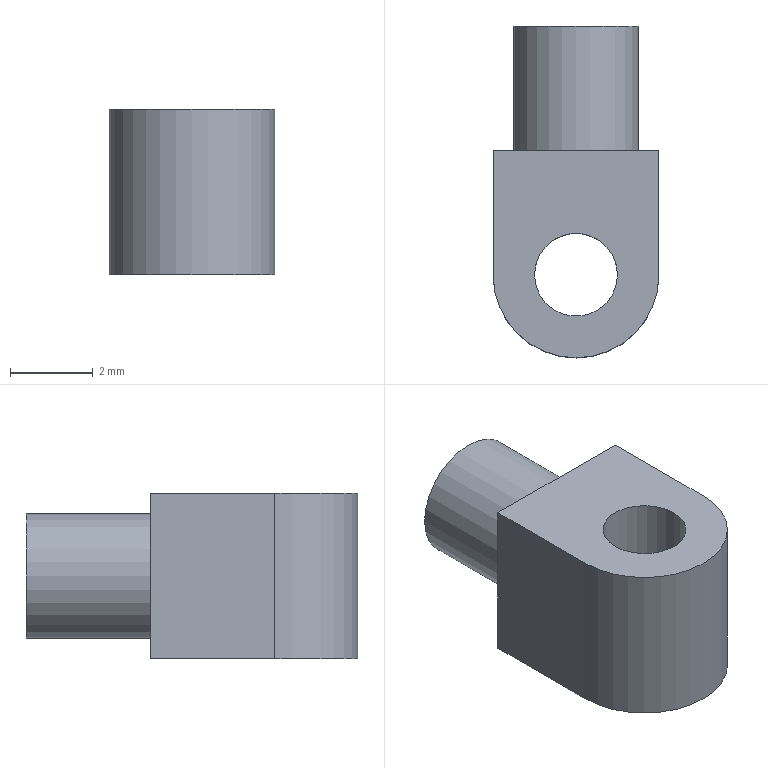Part | STEP file | 1-56.20 | 1 solid | 9 faces | box 4 x 8 x 4 mm | volume 81.772 mm3 | plane 6 | cylinder 3 | commonest cylinder face diameters 2 x1 3 x1 4 x1
STEP:
#1=CARTESIAN_POINT('',(0.,0.,0.));
#2=DIRECTION('',(0.,0.,1.));
#3=DIRECTION('',(1.,0.,0.));
#4=AXIS2_PLACEMENT_3D('',#1,#2,#3);
#5=CARTESIAN_POINT('',(1.5,3.,0.));
#6=VERTEX_POINT('',#5);
#7=CARTESIAN_POINT('',(0.,3.,0.));
#8=DIRECTION('',(0.,-1.,0.));
#9=DIRECTION('',(1.,0.,0.));
#10=AXIS2_PLACEMENT_3D('',#7,#8,#9);
#11=CIRCLE('',#10,1.5);
#12=CARTESIAN_POINT('',(-0.4019,3.,0.));
#13=DIRECTION('',(0.,-1.,0.));
#14=DIRECTION('',(1.,0.,0.));
#15=AXIS2_PLACEMENT_3D('',#12,#13,#14);
#16=PLANE('',#15);
#17=CARTESIAN_POINT('',(0.4019,0.));
#18=DIRECTION('',(1.,0.));
#19=AXIS2_PLACEMENT_2D('',#17,#18);
#20=CIRCLE('',#19,1.5);
#21=(GEOMETRIC_REPRESENTATION_CONTEXT(2)PARAMETRIC_REPRESENTATION_CONTEXT()REPRESENTATION_CONTEXT('',''));
#22=DEFINITIONAL_REPRESENTATION('',(#20),#21);
#23=PCURVE('',#16,#22);
#24=CARTESIAN_POINT('',(0.,0.,0.));
#25=DIRECTION('',(0.,1.,0.));
#26=DIRECTION('',(1.,0.,0.));
#27=AXIS2_PLACEMENT_3D('',#24,#25,#26);
#28=CYLINDRICAL_SURFACE('',#27,1.5);
#29=CARTESIAN_POINT('',(6.283,3.));
#30=DIRECTION('',(-1.,0.));
#31=VECTOR('',#30,1.);
#32=LINE('',#29,#31);
#33=(GEOMETRIC_REPRESENTATION_CONTEXT(2)PARAMETRIC_REPRESENTATION_CONTEXT()REPRESENTATION_CONTEXT('',''));
#34=DEFINITIONAL_REPRESENTATION('',(#32),#33);
#35=PCURVE('',#28,#34);
#36=SURFACE_CURVE('',#11,(#23,#35),.PCURVE_S1.);
#37=EDGE_CURVE('',#6,#6,#36,.T.);
#38=ORIENTED_EDGE('',*,*,#37,.T.);
#39=EDGE_LOOP('',(#38));
#40=FACE_BOUND('',#39,.F.);
#41=ADVANCED_FACE('',(#40),#16,.F.);
#42=CARTESIAN_POINT('',(1.5,0.,0.));
#43=VERTEX_POINT('',#42);
#44=CARTESIAN_POINT('',(1.5,0.,0.));
#45=DIRECTION('',(0.,1.,0.));
#46=VECTOR('',#45,1.);
#47=LINE('',#44,#46);
#48=CARTESIAN_POINT('',(6.283,0.));
#49=DIRECTION('',(0.,1.));
#50=VECTOR('',#49,1.);
#51=LINE('',#48,#50);
#52=(GEOMETRIC_REPRESENTATION_CONTEXT(2)PARAMETRIC_REPRESENTATION_CONTEXT()REPRESENTATION_CONTEXT('',''));
#53=DEFINITIONAL_REPRESENTATION('',(#51),#52);
#54=PCURVE('',#28,#53);
#55=CARTESIAN_POINT('',(0.,0.));
#56=DIRECTION('',(0.,1.));
#57=VECTOR('',#56,1.);
#58=LINE('',#55,#57);
#59=(GEOMETRIC_REPRESENTATION_CONTEXT(2)PARAMETRIC_REPRESENTATION_CONTEXT()REPRESENTATION_CONTEXT('',''));
#60=DEFINITIONAL_REPRESENTATION('',(#58),#59);
#61=PCURVE('',#28,#60);
#62=SEAM_CURVE('',#47,(#54,#61),.PCURVE_S1.);
#63=EDGE_CURVE('',#43,#6,#62,.T.);
#64=ORIENTED_EDGE('',*,*,#63,.T.);
#65=ORIENTED_EDGE('',*,*,#37,.T.);
#66=ORIENTED_EDGE('',*,*,#63,.F.);
#67=CARTESIAN_POINT('',(0.,0.,0.));
#68=DIRECTION('',(0.,-1.,0.));
#69=DIRECTION('',(1.,0.,0.));
#70=AXIS2_PLACEMENT_3D('',#67,#68,#69);
#71=CIRCLE('',#70,1.5);
#72=CARTESIAN_POINT('',(6.283,0.));
#73=DIRECTION('',(-1.,0.));
#74=VECTOR('',#73,1.);
#75=LINE('',#72,#74);
#76=(GEOMETRIC_REPRESENTATION_CONTEXT(2)PARAMETRIC_REPRESENTATION_CONTEXT()REPRESENTATION_CONTEXT('',''));
#77=DEFINITIONAL_REPRESENTATION('',(#75),#76);
#78=PCURVE('',#28,#77);
#79=CARTESIAN_POINT('',(0.,0.,0.));
#80=DIRECTION('',(0.,-1.,0.));
#81=DIRECTION('',(-1.,0.,0.));
#82=AXIS2_PLACEMENT_3D('',#79,#80,#81);
#83=PLANE('',#82);
#84=CARTESIAN_POINT('',(0.,0.));
#85=DIRECTION('',(-1.,0.));
#86=AXIS2_PLACEMENT_2D('',#84,#85);
#87=CIRCLE('',#86,1.5);
#88=(GEOMETRIC_REPRESENTATION_CONTEXT(2)PARAMETRIC_REPRESENTATION_CONTEXT()REPRESENTATION_CONTEXT('',''));
#89=DEFINITIONAL_REPRESENTATION('',(#87),#88);
#90=PCURVE('',#83,#89);
#91=SURFACE_CURVE('',#71,(#78,#90),.PCURVE_S1.);
#92=EDGE_CURVE('',#43,#43,#91,.T.);
#93=ORIENTED_EDGE('',*,*,#92,.F.);
#94=EDGE_LOOP('',(#64,#65,#66,#93));
#95=FACE_BOUND('',#94,.T.);
#96=ADVANCED_FACE('',(#95),#28,.T.);
#97=CARTESIAN_POINT('',(2.,0.,2.));
#98=VERTEX_POINT('',#97);
#99=CARTESIAN_POINT('',(-2.,0.,2.));
#100=VERTEX_POINT('',#99);
#101=CARTESIAN_POINT('',(2.,0.,2.));
#102=DIRECTION('',(-1.,0.,0.));
#103=VECTOR('',#102,1.);
#104=LINE('',#101,#103);
#105=CARTESIAN_POINT('',(-2.,-2.));
#106=DIRECTION('',(1.,0.));
#107=VECTOR('',#106,1.);
#108=LINE('',#105,#107);
#109=(GEOMETRIC_REPRESENTATION_CONTEXT(2)PARAMETRIC_REPRESENTATION_CONTEXT()REPRESENTATION_CONTEXT('',''));
#110=DEFINITIONAL_REPRESENTATION('',(#108),#109);
#111=PCURVE('',#83,#110);
#112=CARTESIAN_POINT('',(0.5,-2.5,2.));
#113=DIRECTION('',(0.,0.,1.));
#114=DIRECTION('',(1.,0.,0.));
#115=AXIS2_PLACEMENT_3D('',#112,#113,#114);
#116=PLANE('',#115);
#117=CARTESIAN_POINT('',(1.5,2.5));
#118=DIRECTION('',(-1.,0.));
#119=VECTOR('',#118,1.);
#120=LINE('',#117,#119);
#121=(GEOMETRIC_REPRESENTATION_CONTEXT(2)PARAMETRIC_REPRESENTATION_CONTEXT()REPRESENTATION_CONTEXT('',''));
#122=DEFINITIONAL_REPRESENTATION('',(#120),#121);
#123=PCURVE('',#116,#122);
#124=SURFACE_CURVE('',#104,(#111,#123),.PCURVE_S1.);
#125=EDGE_CURVE('',#98,#100,#124,.T.);
#126=ORIENTED_EDGE('',*,*,#125,.T.);
#127=CARTESIAN_POINT('',(-2.,0.,-2.));
#128=VERTEX_POINT('',#127);
#129=CARTESIAN_POINT('',(-2.,0.,2.));
#130=DIRECTION('',(0.,0.,-1.));
#131=VECTOR('',#130,1.);
#132=LINE('',#129,#131);
#133=CARTESIAN_POINT('',(2.,-2.));
#134=DIRECTION('',(0.,1.));
#135=VECTOR('',#134,1.);
#136=LINE('',#133,#135);
#137=(GEOMETRIC_REPRESENTATION_CONTEXT(2)PARAMETRIC_REPRESENTATION_CONTEXT()REPRESENTATION_CONTEXT('',''));
#138=DEFINITIONAL_REPRESENTATION('',(#136),#137);
#139=PCURVE('',#83,#138);
#140=CARTESIAN_POINT('',(-2.,-1.5,0.));
#141=DIRECTION('',(1.,0.,0.));
#142=DIRECTION('',(0.,-1.,0.));
#143=AXIS2_PLACEMENT_3D('',#140,#141,#142);
#144=PLANE('',#143);
#145=CARTESIAN_POINT('',(-1.5,-2.));
#146=DIRECTION('',(0.,1.));
#147=VECTOR('',#146,1.);
#148=LINE('',#145,#147);
#149=(GEOMETRIC_REPRESENTATION_CONTEXT(2)PARAMETRIC_REPRESENTATION_CONTEXT()REPRESENTATION_CONTEXT('',''));
#150=DEFINITIONAL_REPRESENTATION('',(#148),#149);
#151=PCURVE('',#144,#150);
#152=SURFACE_CURVE('',#132,(#139,#151),.PCURVE_S1.);
#153=EDGE_CURVE('',#100,#128,#152,.T.);
#154=ORIENTED_EDGE('',*,*,#153,.T.);
#155=CARTESIAN_POINT('',(2.,0.,-2.));
#156=VERTEX_POINT('',#155);
#157=CARTESIAN_POINT('',(2.,0.,-2.));
#158=DIRECTION('',(-1.,0.,0.));
#159=VECTOR('',#158,1.);
#160=LINE('',#157,#159);
#161=CARTESIAN_POINT('',(-2.,2.));
#162=DIRECTION('',(1.,0.));
#163=VECTOR('',#162,1.);
#164=LINE('',#161,#163);
#165=(GEOMETRIC_REPRESENTATION_CONTEXT(2)PARAMETRIC_REPRESENTATION_CONTEXT()REPRESENTATION_CONTEXT('',''));
#166=DEFINITIONAL_REPRESENTATION('',(#164),#165);
#167=PCURVE('',#83,#166);
#168=CARTESIAN_POINT('',(0.5,-2.5,-2.));
#169=DIRECTION('',(0.,0.,1.));
#170=DIRECTION('',(1.,0.,0.));
#171=AXIS2_PLACEMENT_3D('',#168,#169,#170);
#172=PLANE('',#171);
#173=CARTESIAN_POINT('',(1.5,2.5));
#174=DIRECTION('',(-1.,0.));
#175=VECTOR('',#174,1.);
#176=LINE('',#173,#175);
#177=(GEOMETRIC_REPRESENTATION_CONTEXT(2)PARAMETRIC_REPRESENTATION_CONTEXT()REPRESENTATION_CONTEXT('',''));
#178=DEFINITIONAL_REPRESENTATION('',(#176),#177);
#179=PCURVE('',#172,#178);
#180=SURFACE_CURVE('',#160,(#167,#179),.PCURVE_S1.);
#181=EDGE_CURVE('',#156,#128,#180,.T.);
#182=ORIENTED_EDGE('',*,*,#181,.F.);
#183=CARTESIAN_POINT('',(2.,0.,2.));
#184=DIRECTION('',(0.,0.,-1.));
#185=VECTOR('',#184,1.);
#186=LINE('',#183,#185);
#187=CARTESIAN_POINT('',(-2.,-2.));
#188=DIRECTION('',(0.,1.));
#189=VECTOR('',#188,1.);
#190=LINE('',#187,#189);
#191=(GEOMETRIC_REPRESENTATION_CONTEXT(2)PARAMETRIC_REPRESENTATION_CONTEXT()REPRESENTATION_CONTEXT('',''));
#192=DEFINITIONAL_REPRESENTATION('',(#190),#191);
#193=PCURVE('',#83,#192);
#194=CARTESIAN_POINT('',(2.,-1.5,0.));
#195=DIRECTION('',(-1.,0.,0.));
#196=DIRECTION('',(0.,1.,0.));
#197=AXIS2_PLACEMENT_3D('',#194,#195,#196);
#198=PLANE('',#197);
#199=CARTESIAN_POINT('',(1.5,-2.));
#200=DIRECTION('',(0.,1.));
#201=VECTOR('',#200,1.);
#202=LINE('',#199,#201);
#203=(GEOMETRIC_REPRESENTATION_CONTEXT(2)PARAMETRIC_REPRESENTATION_CONTEXT()REPRESENTATION_CONTEXT('',''));
#204=DEFINITIONAL_REPRESENTATION('',(#202),#203);
#205=PCURVE('',#198,#204);
#206=SURFACE_CURVE('',#186,(#193,#205),.PCURVE_S1.);
#207=EDGE_CURVE('',#98,#156,#206,.T.);
#208=ORIENTED_EDGE('',*,*,#207,.F.);
#209=EDGE_LOOP('',(#126,#154,#182,#208));
#210=FACE_BOUND('',#209,.F.);
#211=ORIENTED_EDGE('',*,*,#92,.F.);
#212=EDGE_LOOP('',(#211));
#213=FACE_BOUND('',#212,.F.);
#214=ADVANCED_FACE('',(#210,#213),#83,.F.);
#215=ORIENTED_EDGE('',*,*,#125,.T.);
#216=CARTESIAN_POINT('',(-2.,-3.,2.));
#217=VERTEX_POINT('',#216);
#218=CARTESIAN_POINT('',(-2.,0.,2.));
#219=DIRECTION('',(0.,-1.,0.));
#220=VECTOR('',#219,1.);
#221=LINE('',#218,#220);
#222=CARTESIAN_POINT('',(-2.5,2.5));
#223=DIRECTION('',(0.,-1.));
#224=VECTOR('',#223,1.);
#225=LINE('',#222,#224);
#226=(GEOMETRIC_REPRESENTATION_CONTEXT(2)PARAMETRIC_REPRESENTATION_CONTEXT()REPRESENTATION_CONTEXT('',''));
#227=DEFINITIONAL_REPRESENTATION('',(#225),#226);
#228=PCURVE('',#116,#227);
#229=CARTESIAN_POINT('',(-1.5,-2.));
#230=DIRECTION('',(1.,0.));
#231=VECTOR('',#230,1.);
#232=LINE('',#229,#231);
#233=(GEOMETRIC_REPRESENTATION_CONTEXT(2)PARAMETRIC_REPRESENTATION_CONTEXT()REPRESENTATION_CONTEXT('',''));
#234=DEFINITIONAL_REPRESENTATION('',(#232),#233);
#235=PCURVE('',#144,#234);
#236=SURFACE_CURVE('',#221,(#228,#235),.PCURVE_S1.);
#237=EDGE_CURVE('',#100,#217,#236,.T.);
#238=ORIENTED_EDGE('',*,*,#237,.T.);
#239=CARTESIAN_POINT('',(2.,-3.,2.));
#240=VERTEX_POINT('',#239);
#241=CARTESIAN_POINT('',(0.,-3.,2.));
#242=DIRECTION('',(0.,0.,1.));
#243=DIRECTION('',(-1.,0.,0.));
#244=AXIS2_PLACEMENT_3D('',#241,#242,#243);
#245=CIRCLE('',#244,2.);
#246=CARTESIAN_POINT('',(-0.5,-0.5));
#247=DIRECTION('',(-1.,0.));
#248=AXIS2_PLACEMENT_2D('',#246,#247);
#249=CIRCLE('',#248,2.);
#250=(GEOMETRIC_REPRESENTATION_CONTEXT(2)PARAMETRIC_REPRESENTATION_CONTEXT()REPRESENTATION_CONTEXT('',''));
#251=DEFINITIONAL_REPRESENTATION('',(#249),#250);
#252=PCURVE('',#116,#251);
#253=CARTESIAN_POINT('',(0.,-3.,2.));
#254=DIRECTION('',(0.,0.,-1.));
#255=DIRECTION('',(-1.,0.,0.));
#256=AXIS2_PLACEMENT_3D('',#253,#254,#255);
#257=CYLINDRICAL_SURFACE('',#256,2.);
#258=CARTESIAN_POINT('',(6.283,0.));
#259=DIRECTION('',(-1.,0.));
#260=VECTOR('',#259,1.);
#261=LINE('',#258,#260);
#262=(GEOMETRIC_REPRESENTATION_CONTEXT(2)PARAMETRIC_REPRESENTATION_CONTEXT()REPRESENTATION_CONTEXT('',''));
#263=DEFINITIONAL_REPRESENTATION('',(#261),#262);
#264=PCURVE('',#257,#263);
#265=SURFACE_CURVE('',#245,(#252,#264),.PCURVE_S1.);
#266=EDGE_CURVE('',#217,#240,#265,.T.);
#267=ORIENTED_EDGE('',*,*,#266,.T.);
#268=CARTESIAN_POINT('',(2.,-3.,2.));
#269=DIRECTION('',(0.,1.,0.));
#270=VECTOR('',#269,1.);
#271=LINE('',#268,#270);
#272=CARTESIAN_POINT('',(1.5,-0.5));
#273=DIRECTION('',(0.,1.));
#274=VECTOR('',#273,1.);
#275=LINE('',#272,#274);
#276=(GEOMETRIC_REPRESENTATION_CONTEXT(2)PARAMETRIC_REPRESENTATION_CONTEXT()REPRESENTATION_CONTEXT('',''));
#277=DEFINITIONAL_REPRESENTATION('',(#275),#276);
#278=PCURVE('',#116,#277);
#279=CARTESIAN_POINT('',(-1.5,-2.));
#280=DIRECTION('',(1.,0.));
#281=VECTOR('',#280,1.);
#282=LINE('',#279,#281);
#283=(GEOMETRIC_REPRESENTATION_CONTEXT(2)PARAMETRIC_REPRESENTATION_CONTEXT()REPRESENTATION_CONTEXT('',''));
#284=DEFINITIONAL_REPRESENTATION('',(#282),#283);
#285=PCURVE('',#198,#284);
#286=SURFACE_CURVE('',#271,(#278,#285),.PCURVE_S1.);
#287=EDGE_CURVE('',#240,#98,#286,.T.);
#288=ORIENTED_EDGE('',*,*,#287,.T.);
#289=EDGE_LOOP('',(#215,#238,#267,#288));
#290=FACE_BOUND('',#289,.T.);
#291=CARTESIAN_POINT('',(1.,-3.,2.));
#292=VERTEX_POINT('',#291);
#293=CARTESIAN_POINT('',(0.,-3.,2.));
#294=DIRECTION('',(0.,0.,-1.));
#295=DIRECTION('',(1.,0.,0.));
#296=AXIS2_PLACEMENT_3D('',#293,#294,#295);
#297=CIRCLE('',#296,1.);
#298=CARTESIAN_POINT('',(0.5,-0.5));
#299=CARTESIAN_POINT('',(0.5,-2.232));
#300=CARTESIAN_POINT('',(-1.,-1.366));
#301=CARTESIAN_POINT('',(-2.5,-0.5));
#302=CARTESIAN_POINT('',(-1.,0.366));
#303=CARTESIAN_POINT('',(0.5,1.232));
#304=CARTESIAN_POINT('',(0.5,-0.5));
#305=(BOUNDED_CURVE()B_SPLINE_CURVE(2,(#298,#299,#300,#301,#302,#303,#304),.UNSPECIFIED.,.T.,.F.)B_SPLINE_CURVE_WITH_KNOTS((1,2,2,2,2,1),(-2.094,0.,2.094,4.189,6.283,8.378),.UNSPECIFIED.)CURVE()GEOMETRIC_REPRESENTATION_ITEM()RATIONAL_B_SPLINE_CURVE((1.,0.5,1.,0.5,1.,0.5,1.))REPRESENTATION_ITEM(''));
#306=(GEOMETRIC_REPRESENTATION_CONTEXT(2)PARAMETRIC_REPRESENTATION_CONTEXT()REPRESENTATION_CONTEXT('',''));
#307=DEFINITIONAL_REPRESENTATION('',(#305),#306);
#308=PCURVE('',#116,#307);
#309=CARTESIAN_POINT('',(0.,-3.,2.));
#310=DIRECTION('',(0.,0.,-1.));
#311=DIRECTION('',(1.,0.,0.));
#312=AXIS2_PLACEMENT_3D('',#309,#310,#311);
#313=CYLINDRICAL_SURFACE('',#312,1.);
#314=CARTESIAN_POINT('',(0.,0.));
#315=DIRECTION('',(1.,0.));
#316=VECTOR('',#315,1.);
#317=LINE('',#314,#316);
#318=(GEOMETRIC_REPRESENTATION_CONTEXT(2)PARAMETRIC_REPRESENTATION_CONTEXT()REPRESENTATION_CONTEXT('',''));
#319=DEFINITIONAL_REPRESENTATION('',(#317),#318);
#320=PCURVE('',#313,#319);
#321=SURFACE_CURVE('',#297,(#308,#320),.PCURVE_S1.);
#322=EDGE_CURVE('',#292,#292,#321,.T.);
#323=ORIENTED_EDGE('',*,*,#322,.T.);
#324=EDGE_LOOP('',(#323));
#325=FACE_BOUND('',#324,.T.);
#326=ADVANCED_FACE('',(#290,#325),#116,.T.);
#327=ORIENTED_EDGE('',*,*,#181,.T.);
#328=CARTESIAN_POINT('',(-2.,-3.,-2.));
#329=VERTEX_POINT('',#328);
#330=CARTESIAN_POINT('',(-2.,0.,-2.));
#331=DIRECTION('',(0.,-1.,0.));
#332=VECTOR('',#331,1.);
#333=LINE('',#330,#332);
#334=CARTESIAN_POINT('',(-2.5,2.5));
#335=DIRECTION('',(0.,-1.));
#336=VECTOR('',#335,1.);
#337=LINE('',#334,#336);
#338=(GEOMETRIC_REPRESENTATION_CONTEXT(2)PARAMETRIC_REPRESENTATION_CONTEXT()REPRESENTATION_CONTEXT('',''));
#339=DEFINITIONAL_REPRESENTATION('',(#337),#338);
#340=PCURVE('',#172,#339);
#341=CARTESIAN_POINT('',(-1.5,2.));
#342=DIRECTION('',(1.,0.));
#343=VECTOR('',#342,1.);
#344=LINE('',#341,#343);
#345=(GEOMETRIC_REPRESENTATION_CONTEXT(2)PARAMETRIC_REPRESENTATION_CONTEXT()REPRESENTATION_CONTEXT('',''));
#346=DEFINITIONAL_REPRESENTATION('',(#344),#345);
#347=PCURVE('',#144,#346);
#348=SURFACE_CURVE('',#333,(#340,#347),.PCURVE_S1.);
#349=EDGE_CURVE('',#128,#329,#348,.T.);
#350=ORIENTED_EDGE('',*,*,#349,.T.);
#351=CARTESIAN_POINT('',(2.,-3.,-2.));
#352=VERTEX_POINT('',#351);
#353=CARTESIAN_POINT('',(0.,-3.,-2.));
#354=DIRECTION('',(0.,0.,1.));
#355=DIRECTION('',(-1.,0.,0.));
#356=AXIS2_PLACEMENT_3D('',#353,#354,#355);
#357=CIRCLE('',#356,2.);
#358=CARTESIAN_POINT('',(-0.5,-0.5));
#359=DIRECTION('',(-1.,0.));
#360=AXIS2_PLACEMENT_2D('',#358,#359);
#361=CIRCLE('',#360,2.);
#362=(GEOMETRIC_REPRESENTATION_CONTEXT(2)PARAMETRIC_REPRESENTATION_CONTEXT()REPRESENTATION_CONTEXT('',''));
#363=DEFINITIONAL_REPRESENTATION('',(#361),#362);
#364=PCURVE('',#172,#363);
#365=CARTESIAN_POINT('',(6.283,4.));
#366=DIRECTION('',(-1.,0.));
#367=VECTOR('',#366,1.);
#368=LINE('',#365,#367);
#369=(GEOMETRIC_REPRESENTATION_CONTEXT(2)PARAMETRIC_REPRESENTATION_CONTEXT()REPRESENTATION_CONTEXT('',''));
#370=DEFINITIONAL_REPRESENTATION('',(#368),#369);
#371=PCURVE('',#257,#370);
#372=SURFACE_CURVE('',#357,(#364,#371),.PCURVE_S1.);
#373=EDGE_CURVE('',#329,#352,#372,.T.);
#374=ORIENTED_EDGE('',*,*,#373,.T.);
#375=CARTESIAN_POINT('',(2.,-3.,-2.));
#376=DIRECTION('',(0.,1.,0.));
#377=VECTOR('',#376,1.);
#378=LINE('',#375,#377);
#379=CARTESIAN_POINT('',(1.5,-0.5));
#380=DIRECTION('',(0.,1.));
#381=VECTOR('',#380,1.);
#382=LINE('',#379,#381);
#383=(GEOMETRIC_REPRESENTATION_CONTEXT(2)PARAMETRIC_REPRESENTATION_CONTEXT()REPRESENTATION_CONTEXT('',''));
#384=DEFINITIONAL_REPRESENTATION('',(#382),#383);
#385=PCURVE('',#172,#384);
#386=CARTESIAN_POINT('',(-1.5,2.));
#387=DIRECTION('',(1.,0.));
#388=VECTOR('',#387,1.);
#389=LINE('',#386,#388);
#390=(GEOMETRIC_REPRESENTATION_CONTEXT(2)PARAMETRIC_REPRESENTATION_CONTEXT()REPRESENTATION_CONTEXT('',''));
#391=DEFINITIONAL_REPRESENTATION('',(#389),#390);
#392=PCURVE('',#198,#391);
#393=SURFACE_CURVE('',#378,(#385,#392),.PCURVE_S1.);
#394=EDGE_CURVE('',#352,#156,#393,.T.);
#395=ORIENTED_EDGE('',*,*,#394,.T.);
#396=EDGE_LOOP('',(#327,#350,#374,#395));
#397=FACE_BOUND('',#396,.F.);
#398=CARTESIAN_POINT('',(1.,-3.,-2.));
#399=VERTEX_POINT('',#398);
#400=CARTESIAN_POINT('',(0.,-3.,-2.));
#401=DIRECTION('',(0.,0.,-1.));
#402=DIRECTION('',(1.,0.,0.));
#403=AXIS2_PLACEMENT_3D('',#400,#401,#402);
#404=CIRCLE('',#403,1.);
#405=CARTESIAN_POINT('',(0.5,-0.5));
#406=CARTESIAN_POINT('',(0.5,-2.232));
#407=CARTESIAN_POINT('',(-1.,-1.366));
#408=CARTESIAN_POINT('',(-2.5,-0.5));
#409=CARTESIAN_POINT('',(-1.,0.366));
#410=CARTESIAN_POINT('',(0.5,1.232));
#411=CARTESIAN_POINT('',(0.5,-0.5));
#412=(BOUNDED_CURVE()B_SPLINE_CURVE(2,(#405,#406,#407,#408,#409,#410,#411),.UNSPECIFIED.,.T.,.F.)B_SPLINE_CURVE_WITH_KNOTS((1,2,2,2,2,1),(-2.094,0.,2.094,4.189,6.283,8.378),.UNSPECIFIED.)CURVE()GEOMETRIC_REPRESENTATION_ITEM()RATIONAL_B_SPLINE_CURVE((1.,0.5,1.,0.5,1.,0.5,1.))REPRESENTATION_ITEM(''));
#413=(GEOMETRIC_REPRESENTATION_CONTEXT(2)PARAMETRIC_REPRESENTATION_CONTEXT()REPRESENTATION_CONTEXT('',''));
#414=DEFINITIONAL_REPRESENTATION('',(#412),#413);
#415=PCURVE('',#172,#414);
#416=CARTESIAN_POINT('',(0.,4.));
#417=DIRECTION('',(1.,0.));
#418=VECTOR('',#417,1.);
#419=LINE('',#416,#418);
#420=(GEOMETRIC_REPRESENTATION_CONTEXT(2)PARAMETRIC_REPRESENTATION_CONTEXT()REPRESENTATION_CONTEXT('',''));
#421=DEFINITIONAL_REPRESENTATION('',(#419),#420);
#422=PCURVE('',#313,#421);
#423=SURFACE_CURVE('',#404,(#415,#422),.PCURVE_S1.);
#424=EDGE_CURVE('',#399,#399,#423,.T.);
#425=ORIENTED_EDGE('',*,*,#424,.T.);
#426=EDGE_LOOP('',(#425));
#427=FACE_BOUND('',#426,.F.);
#428=ADVANCED_FACE('',(#397,#427),#172,.F.);
#429=ORIENTED_EDGE('',*,*,#237,.T.);
#430=CARTESIAN_POINT('',(-2.,-3.,2.));
#431=DIRECTION('',(0.,0.,-1.));
#432=VECTOR('',#431,1.);
#433=LINE('',#430,#432);
#434=CARTESIAN_POINT('',(1.5,-2.));
#435=DIRECTION('',(0.,1.));
#436=VECTOR('',#435,1.);
#437=LINE('',#434,#436);
#438=(GEOMETRIC_REPRESENTATION_CONTEXT(2)PARAMETRIC_REPRESENTATION_CONTEXT()REPRESENTATION_CONTEXT('',''));
#439=DEFINITIONAL_REPRESENTATION('',(#437),#438);
#440=PCURVE('',#144,#439);
#441=CARTESIAN_POINT('',(6.283,0.));
#442=DIRECTION('',(0.,1.));
#443=VECTOR('',#442,1.);
#444=LINE('',#441,#443);
#445=(GEOMETRIC_REPRESENTATION_CONTEXT(2)PARAMETRIC_REPRESENTATION_CONTEXT()REPRESENTATION_CONTEXT('',''));
#446=DEFINITIONAL_REPRESENTATION('',(#444),#445);
#447=PCURVE('',#257,#446);
#448=SURFACE_CURVE('',#433,(#440,#447),.PCURVE_S1.);
#449=EDGE_CURVE('',#217,#329,#448,.T.);
#450=ORIENTED_EDGE('',*,*,#449,.T.);
#451=ORIENTED_EDGE('',*,*,#349,.F.);
#452=ORIENTED_EDGE('',*,*,#153,.F.);
#453=EDGE_LOOP('',(#429,#450,#451,#452));
#454=FACE_BOUND('',#453,.F.);
#455=ADVANCED_FACE('',(#454),#144,.F.);
#456=ORIENTED_EDGE('',*,*,#287,.T.);
#457=ORIENTED_EDGE('',*,*,#207,.T.);
#458=ORIENTED_EDGE('',*,*,#394,.F.);
#459=CARTESIAN_POINT('',(2.,-3.,2.));
#460=DIRECTION('',(0.,0.,-1.));
#461=VECTOR('',#460,1.);
#462=LINE('',#459,#461);
#463=CARTESIAN_POINT('',(-1.5,-2.));
#464=DIRECTION('',(0.,1.));
#465=VECTOR('',#464,1.);
#466=LINE('',#463,#465);
#467=(GEOMETRIC_REPRESENTATION_CONTEXT(2)PARAMETRIC_REPRESENTATION_CONTEXT()REPRESENTATION_CONTEXT('',''));
#468=DEFINITIONAL_REPRESENTATION('',(#466),#467);
#469=PCURVE('',#198,#468);
#470=CARTESIAN_POINT('',(3.142,0.));
#471=DIRECTION('',(0.,1.));
#472=VECTOR('',#471,1.);
#473=LINE('',#470,#472);
#474=(GEOMETRIC_REPRESENTATION_CONTEXT(2)PARAMETRIC_REPRESENTATION_CONTEXT()REPRESENTATION_CONTEXT('',''));
#475=DEFINITIONAL_REPRESENTATION('',(#473),#474);
#476=PCURVE('',#257,#475);
#477=SURFACE_CURVE('',#462,(#469,#476),.PCURVE_S1.);
#478=EDGE_CURVE('',#240,#352,#477,.T.);
#479=ORIENTED_EDGE('',*,*,#478,.F.);
#480=EDGE_LOOP('',(#456,#457,#458,#479));
#481=FACE_BOUND('',#480,.F.);
#482=ADVANCED_FACE('',(#481),#198,.F.);
#483=ORIENTED_EDGE('',*,*,#449,.T.);
#484=ORIENTED_EDGE('',*,*,#373,.T.);
#485=ORIENTED_EDGE('',*,*,#478,.F.);
#486=ORIENTED_EDGE('',*,*,#266,.F.);
#487=EDGE_LOOP('',(#483,#484,#485,#486));
#488=FACE_BOUND('',#487,.T.);
#489=ADVANCED_FACE('',(#488),#257,.T.);
#490=ORIENTED_EDGE('',*,*,#322,.T.);
#491=CARTESIAN_POINT('',(1.,-3.,2.));
#492=DIRECTION('',(0.,0.,-1.));
#493=VECTOR('',#492,1.);
#494=LINE('',#491,#493);
#495=CARTESIAN_POINT('',(6.283,0.));
#496=DIRECTION('',(0.,1.));
#497=VECTOR('',#496,1.);
#498=LINE('',#495,#497);
#499=(GEOMETRIC_REPRESENTATION_CONTEXT(2)PARAMETRIC_REPRESENTATION_CONTEXT()REPRESENTATION_CONTEXT('',''));
#500=DEFINITIONAL_REPRESENTATION('',(#498),#499);
#501=PCURVE('',#313,#500);
#502=CARTESIAN_POINT('',(0.,0.));
#503=DIRECTION('',(0.,1.));
#504=VECTOR('',#503,1.);
#505=LINE('',#502,#504);
#506=(GEOMETRIC_REPRESENTATION_CONTEXT(2)PARAMETRIC_REPRESENTATION_CONTEXT()REPRESENTATION_CONTEXT('',''));
#507=DEFINITIONAL_REPRESENTATION('',(#505),#506);
#508=PCURVE('',#313,#507);
#509=SEAM_CURVE('',#494,(#501,#508),.PCURVE_S1.);
#510=EDGE_CURVE('',#292,#399,#509,.T.);
#511=ORIENTED_EDGE('',*,*,#510,.T.);
#512=ORIENTED_EDGE('',*,*,#424,.F.);
#513=ORIENTED_EDGE('',*,*,#510,.F.);
#514=EDGE_LOOP('',(#490,#511,#512,#513));
#515=FACE_BOUND('',#514,.F.);
#516=ADVANCED_FACE('',(#515),#313,.F.);
#517=CLOSED_SHELL('',(#41,#96,#214,#326,#428,#455,#482,#489,#516));
#518=MANIFOLD_SOLID_BREP('',#517);
#519=(LENGTH_UNIT()NAMED_UNIT(*)SI_UNIT(.MILLI.,.METRE.));
#520=UNCERTAINTY_MEASURE_WITH_UNIT(LENGTH_MEASURE(0.0000001),#519,'','');
#521=(NAMED_UNIT(*)PLANE_ANGLE_UNIT()SI_UNIT($,.RADIAN.));
#522=(NAMED_UNIT(*)SI_UNIT($,.STERADIAN.)SOLID_ANGLE_UNIT());
#523=(GEOMETRIC_REPRESENTATION_CONTEXT(3)GLOBAL_UNCERTAINTY_ASSIGNED_CONTEXT((#520))GLOBAL_UNIT_ASSIGNED_CONTEXT((#519,#521,#522))REPRESENTATION_CONTEXT('',''));
#524=ADVANCED_BREP_SHAPE_REPRESENTATION('',(#4,#518),#523);